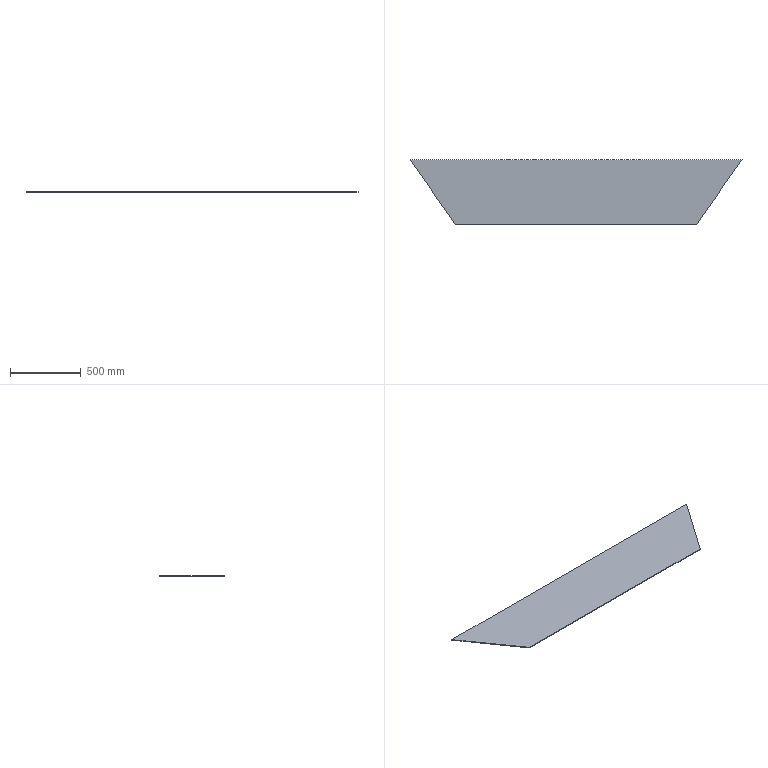Part | SolidWorks | features FlatPattern 1, SMBaseFlange 1, SheetMetal 1 | 1 solid | 6 faces | box 2348 x 455 x 5 mm | volume 4611425 mm3 | plane 6
STEP:
#1=CARTESIAN_POINT('',(0.,0.,0.));
#2=VERTEX_POINT('',#1);
#3=CARTESIAN_POINT('',(1706.,0.,0.));
#4=VERTEX_POINT('',#3);
#5=CARTESIAN_POINT('',(0.,0.,0.));
#6=DIRECTION('',(1.,0.,0.));
#7=VECTOR('',#6,1000.);
#8=LINE('',#5,#7);
#9=EDGE_CURVE('',#2,#4,#8,.T.);
#10=ORIENTED_EDGE('',*,*,#9,.F.);
#11=CARTESIAN_POINT('',(0.,0.,-5.));
#12=VERTEX_POINT('',#11);
#13=CARTESIAN_POINT('',(0.,0.,-5.));
#14=DIRECTION('',(0.,0.,1.));
#15=VECTOR('',#14,1000.);
#16=LINE('',#13,#15);
#17=EDGE_CURVE('',#12,#2,#16,.T.);
#18=ORIENTED_EDGE('',*,*,#17,.F.);
#19=CARTESIAN_POINT('',(1706.,0.,-5.));
#20=VERTEX_POINT('',#19);
#21=CARTESIAN_POINT('',(0.,0.,-5.));
#22=DIRECTION('',(1.,0.,0.));
#23=VECTOR('',#22,1000.);
#24=LINE('',#21,#23);
#25=EDGE_CURVE('',#12,#20,#24,.T.);
#26=ORIENTED_EDGE('',*,*,#25,.T.);
#27=CARTESIAN_POINT('',(1706.,0.,-5.));
#28=DIRECTION('',(0.,0.,1.));
#29=VECTOR('',#28,1000.);
#30=LINE('',#27,#29);
#31=EDGE_CURVE('',#20,#4,#30,.T.);
#32=ORIENTED_EDGE('',*,*,#31,.T.);
#33=EDGE_LOOP('',(#10,#18,#26,#32));
#34=FACE_OUTER_BOUND('',#33,.T.);
#35=CARTESIAN_POINT('',(0.,0.,-5.));
#36=DIRECTION('',(0.,-1.,0.));
#37=DIRECTION('',(0.,0.,-1.));
#38=AXIS2_PLACEMENT_3D('',#35,#36,#37);
#39=PLANE('',#38);
#40=ADVANCED_FACE('',(#34),#39,.T.);
#41=CARTESIAN_POINT('',(-321.,455.,0.));
#42=VERTEX_POINT('',#41);
#43=CARTESIAN_POINT('',(0.,0.,0.));
#44=DIRECTION('',(0.5765,-0.8171,0.));
#45=VECTOR('',#44,1000.);
#46=LINE('',#43,#45);
#47=EDGE_CURVE('',#42,#2,#46,.T.);
#48=ORIENTED_EDGE('',*,*,#47,.F.);
#49=CARTESIAN_POINT('',(-321.,455.,-5.));
#50=VERTEX_POINT('',#49);
#51=CARTESIAN_POINT('',(-321.,455.,-5.));
#52=DIRECTION('',(0.,0.,1.));
#53=VECTOR('',#52,1000.);
#54=LINE('',#51,#53);
#55=EDGE_CURVE('',#50,#42,#54,.T.);
#56=ORIENTED_EDGE('',*,*,#55,.F.);
#57=CARTESIAN_POINT('',(0.,0.,-5.));
#58=DIRECTION('',(0.5765,-0.8171,0.));
#59=VECTOR('',#58,1000.);
#60=LINE('',#57,#59);
#61=EDGE_CURVE('',#50,#12,#60,.T.);
#62=ORIENTED_EDGE('',*,*,#61,.T.);
#63=ORIENTED_EDGE('',*,*,#17,.T.);
#64=EDGE_LOOP('',(#48,#56,#62,#63));
#65=FACE_OUTER_BOUND('',#64,.T.);
#66=CARTESIAN_POINT('',(0.,0.,-5.));
#67=DIRECTION('',(-0.8171,-0.5765,0.));
#68=DIRECTION('',(0.5765,-0.8171,0.));
#69=AXIS2_PLACEMENT_3D('',#66,#67,#68);
#70=PLANE('',#69);
#71=ADVANCED_FACE('',(#65),#70,.T.);
#72=CARTESIAN_POINT('',(2027.,455.,0.));
#73=VERTEX_POINT('',#72);
#74=CARTESIAN_POINT('',(-321.,455.,0.));
#75=DIRECTION('',(-1.,0.,0.));
#76=VECTOR('',#75,1000.);
#77=LINE('',#74,#76);
#78=EDGE_CURVE('',#73,#42,#77,.T.);
#79=ORIENTED_EDGE('',*,*,#78,.F.);
#80=CARTESIAN_POINT('',(2027.,455.,-5.));
#81=VERTEX_POINT('',#80);
#82=CARTESIAN_POINT('',(2027.,455.,-5.));
#83=DIRECTION('',(0.,0.,1.));
#84=VECTOR('',#83,1000.);
#85=LINE('',#82,#84);
#86=EDGE_CURVE('',#81,#73,#85,.T.);
#87=ORIENTED_EDGE('',*,*,#86,.F.);
#88=CARTESIAN_POINT('',(-321.,455.,-5.));
#89=DIRECTION('',(-1.,0.,0.));
#90=VECTOR('',#89,1000.);
#91=LINE('',#88,#90);
#92=EDGE_CURVE('',#81,#50,#91,.T.);
#93=ORIENTED_EDGE('',*,*,#92,.T.);
#94=ORIENTED_EDGE('',*,*,#55,.T.);
#95=EDGE_LOOP('',(#79,#87,#93,#94));
#96=FACE_OUTER_BOUND('',#95,.T.);
#97=CARTESIAN_POINT('',(-321.,455.,-5.));
#98=DIRECTION('',(0.,1.,0.));
#99=DIRECTION('',(0.,0.,1.));
#100=AXIS2_PLACEMENT_3D('',#97,#98,#99);
#101=PLANE('',#100);
#102=ADVANCED_FACE('',(#96),#101,.T.);
#103=CARTESIAN_POINT('',(1706.,0.,0.));
#104=DIRECTION('',(0.5765,0.8171,0.));
#105=VECTOR('',#104,1000.);
#106=LINE('',#103,#105);
#107=EDGE_CURVE('',#4,#73,#106,.T.);
#108=ORIENTED_EDGE('',*,*,#107,.F.);
#109=ORIENTED_EDGE('',*,*,#31,.F.);
#110=CARTESIAN_POINT('',(1706.,0.,-5.));
#111=DIRECTION('',(0.5765,0.8171,0.));
#112=VECTOR('',#111,1000.);
#113=LINE('',#110,#112);
#114=EDGE_CURVE('',#20,#81,#113,.T.);
#115=ORIENTED_EDGE('',*,*,#114,.T.);
#116=ORIENTED_EDGE('',*,*,#86,.T.);
#117=EDGE_LOOP('',(#108,#109,#115,#116));
#118=FACE_OUTER_BOUND('',#117,.T.);
#119=CARTESIAN_POINT('',(1706.,0.,-5.));
#120=DIRECTION('',(0.8171,-0.5765,0.));
#121=DIRECTION('',(0.5765,0.8171,0.));
#122=AXIS2_PLACEMENT_3D('',#119,#120,#121);
#123=PLANE('',#122);
#124=ADVANCED_FACE('',(#118),#123,.T.);
#125=ORIENTED_EDGE('',*,*,#25,.F.);
#126=ORIENTED_EDGE('',*,*,#61,.F.);
#127=ORIENTED_EDGE('',*,*,#92,.F.);
#128=ORIENTED_EDGE('',*,*,#114,.F.);
#129=EDGE_LOOP('',(#125,#126,#127,#128));
#130=FACE_OUTER_BOUND('',#129,.T.);
#131=CARTESIAN_POINT('',(0.,0.,-5.));
#132=DIRECTION('',(0.,0.,1.));
#133=DIRECTION('',(1.,0.,0.));
#134=AXIS2_PLACEMENT_3D('',#131,#132,#133);
#135=PLANE('',#134);
#136=ADVANCED_FACE('',(#130),#135,.F.);
#137=ORIENTED_EDGE('',*,*,#9,.T.);
#138=ORIENTED_EDGE('',*,*,#107,.T.);
#139=ORIENTED_EDGE('',*,*,#78,.T.);
#140=ORIENTED_EDGE('',*,*,#47,.T.);
#141=EDGE_LOOP('',(#137,#138,#139,#140));
#142=FACE_OUTER_BOUND('',#141,.T.);
#143=CARTESIAN_POINT('',(0.,0.,0.));
#144=DIRECTION('',(0.,0.,1.));
#145=DIRECTION('',(1.,0.,0.));
#146=AXIS2_PLACEMENT_3D('',#143,#144,#145);
#147=PLANE('',#146);
#148=ADVANCED_FACE('',(#142),#147,.T.);
#149=CLOSED_SHELL('',(#40,#71,#102,#124,#136,#148));
#150=MANIFOLD_SOLID_BREP('',#149);
#151=CARTESIAN_POINT('',(0.,0.,0.));
#152=DIRECTION('',(0.,0.,1.));
#153=DIRECTION('',(1.,0.,0.));
#154=AXIS2_PLACEMENT_3D('',#151,#152,#153);
#155=(LENGTH_UNIT()NAMED_UNIT(*)SI_UNIT(.MILLI.,.METRE.));
#156=UNCERTAINTY_MEASURE_WITH_UNIT(LENGTH_MEASURE(0.00001),#155,'','');
#157=(NAMED_UNIT(*)PLANE_ANGLE_UNIT()SI_UNIT($,.RADIAN.));
#158=(NAMED_UNIT(*)SI_UNIT($,.STERADIAN.)SOLID_ANGLE_UNIT());
#159=(GEOMETRIC_REPRESENTATION_CONTEXT(3)GLOBAL_UNCERTAINTY_ASSIGNED_CONTEXT((#156))GLOBAL_UNIT_ASSIGNED_CONTEXT((#155,#157,#158))REPRESENTATION_CONTEXT('',''));
#160=ADVANCED_BREP_SHAPE_REPRESENTATION('',(#150,#154),#159);